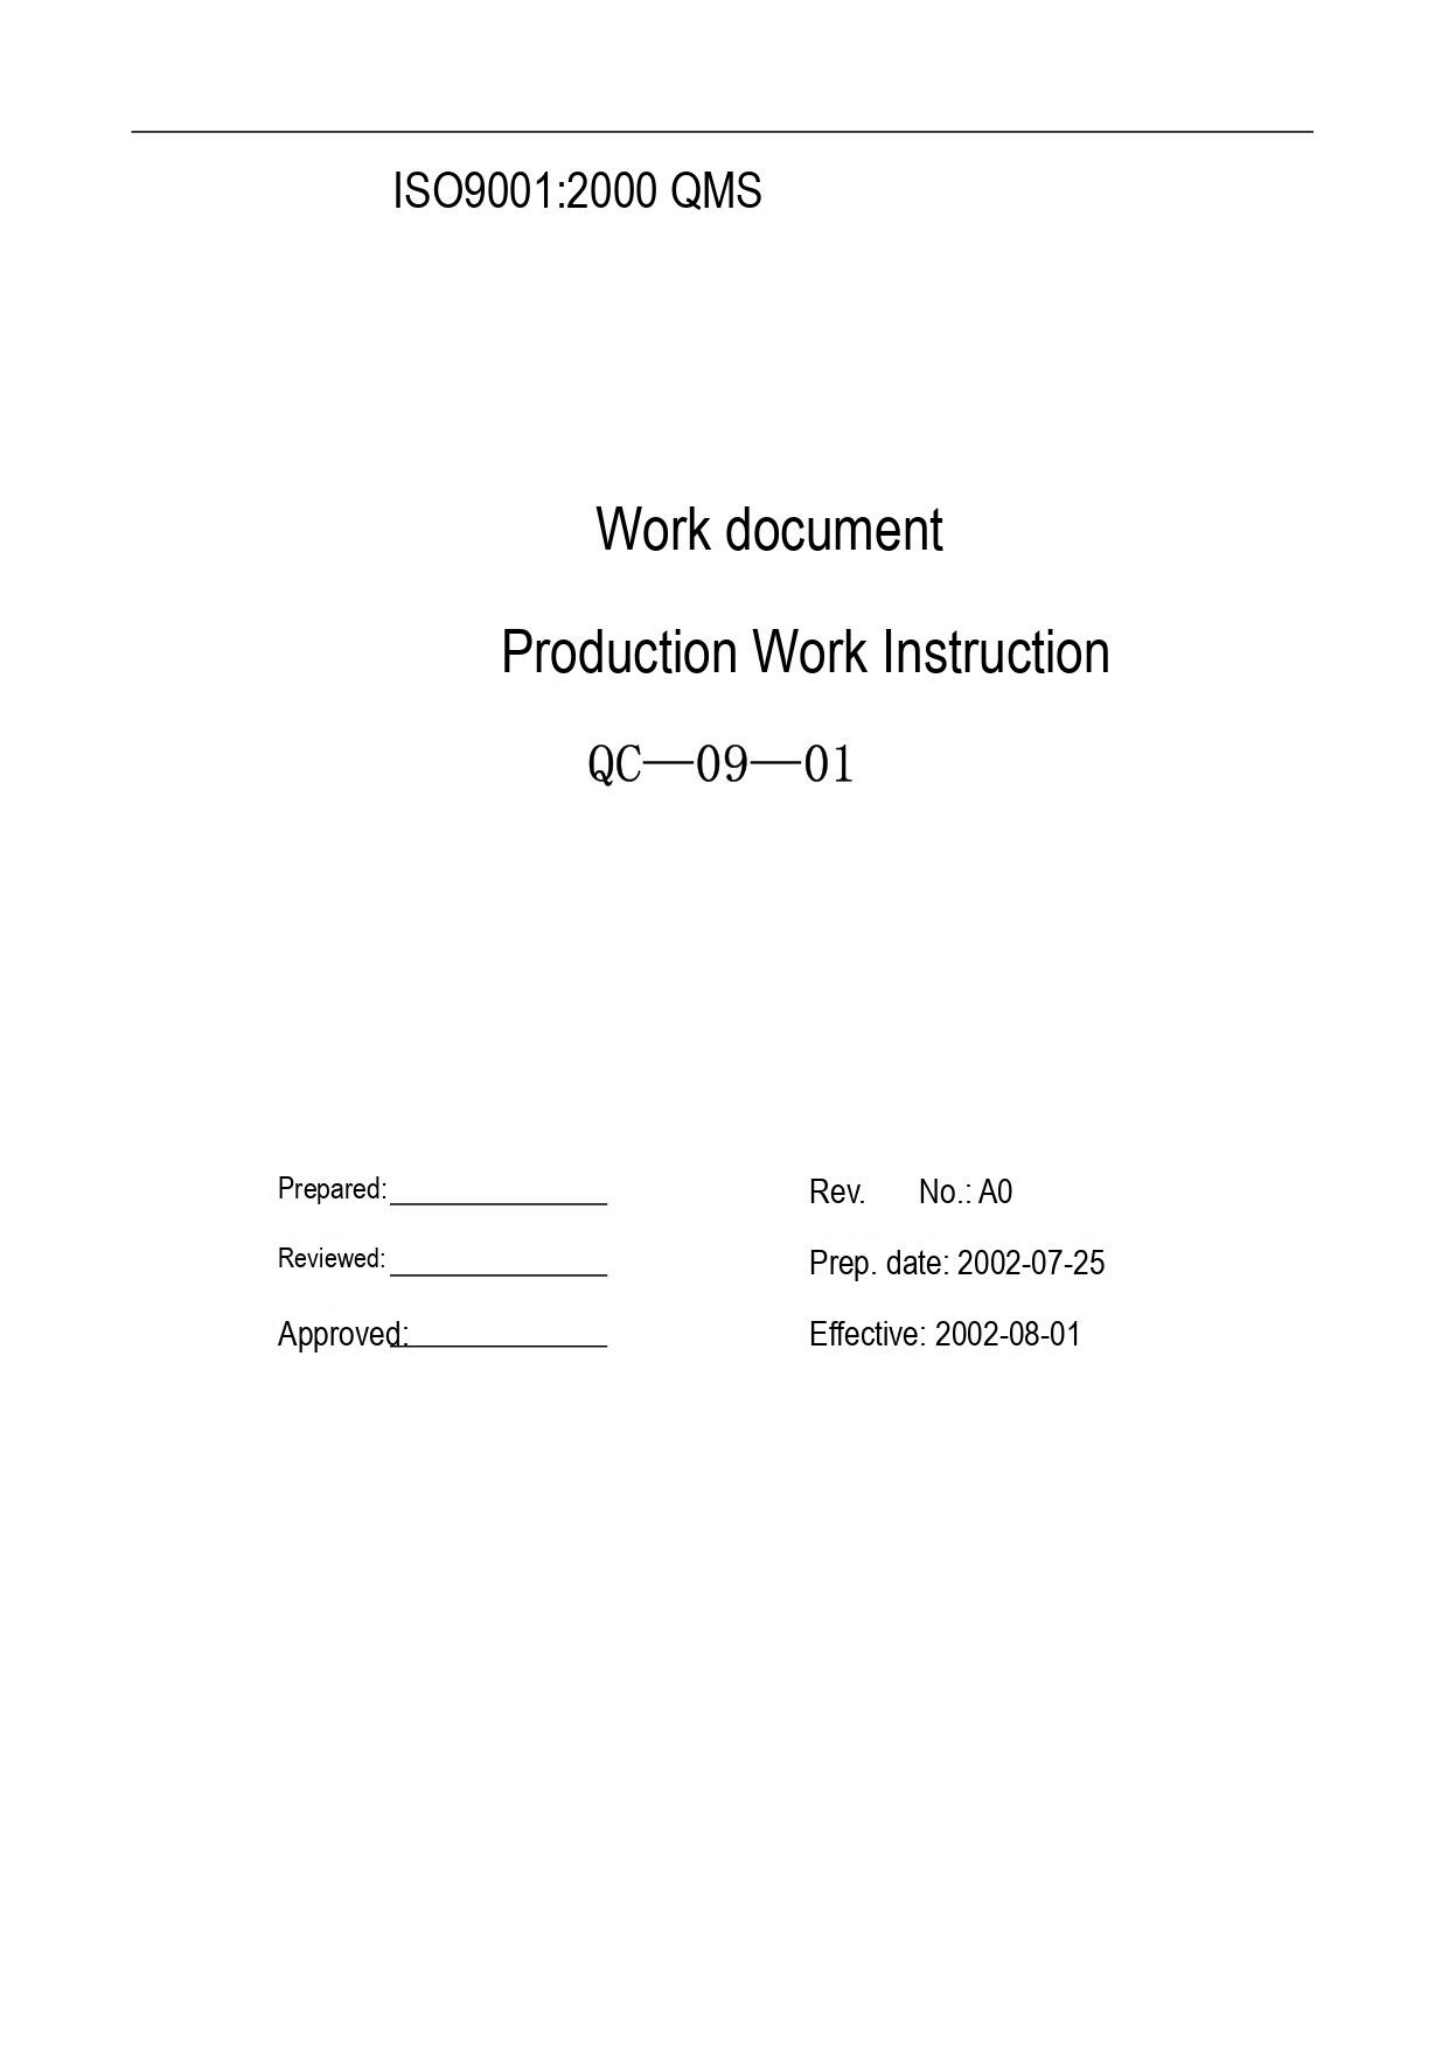ISO9001:2000 QMS

Work document

Production Work Instruction

QC—09—01

Prepared:_______________

Reviewed:_______________

Approved:_______________

Rev. No.: A0

Prep. date: 2002-07-25

Effective: 2002-08-01
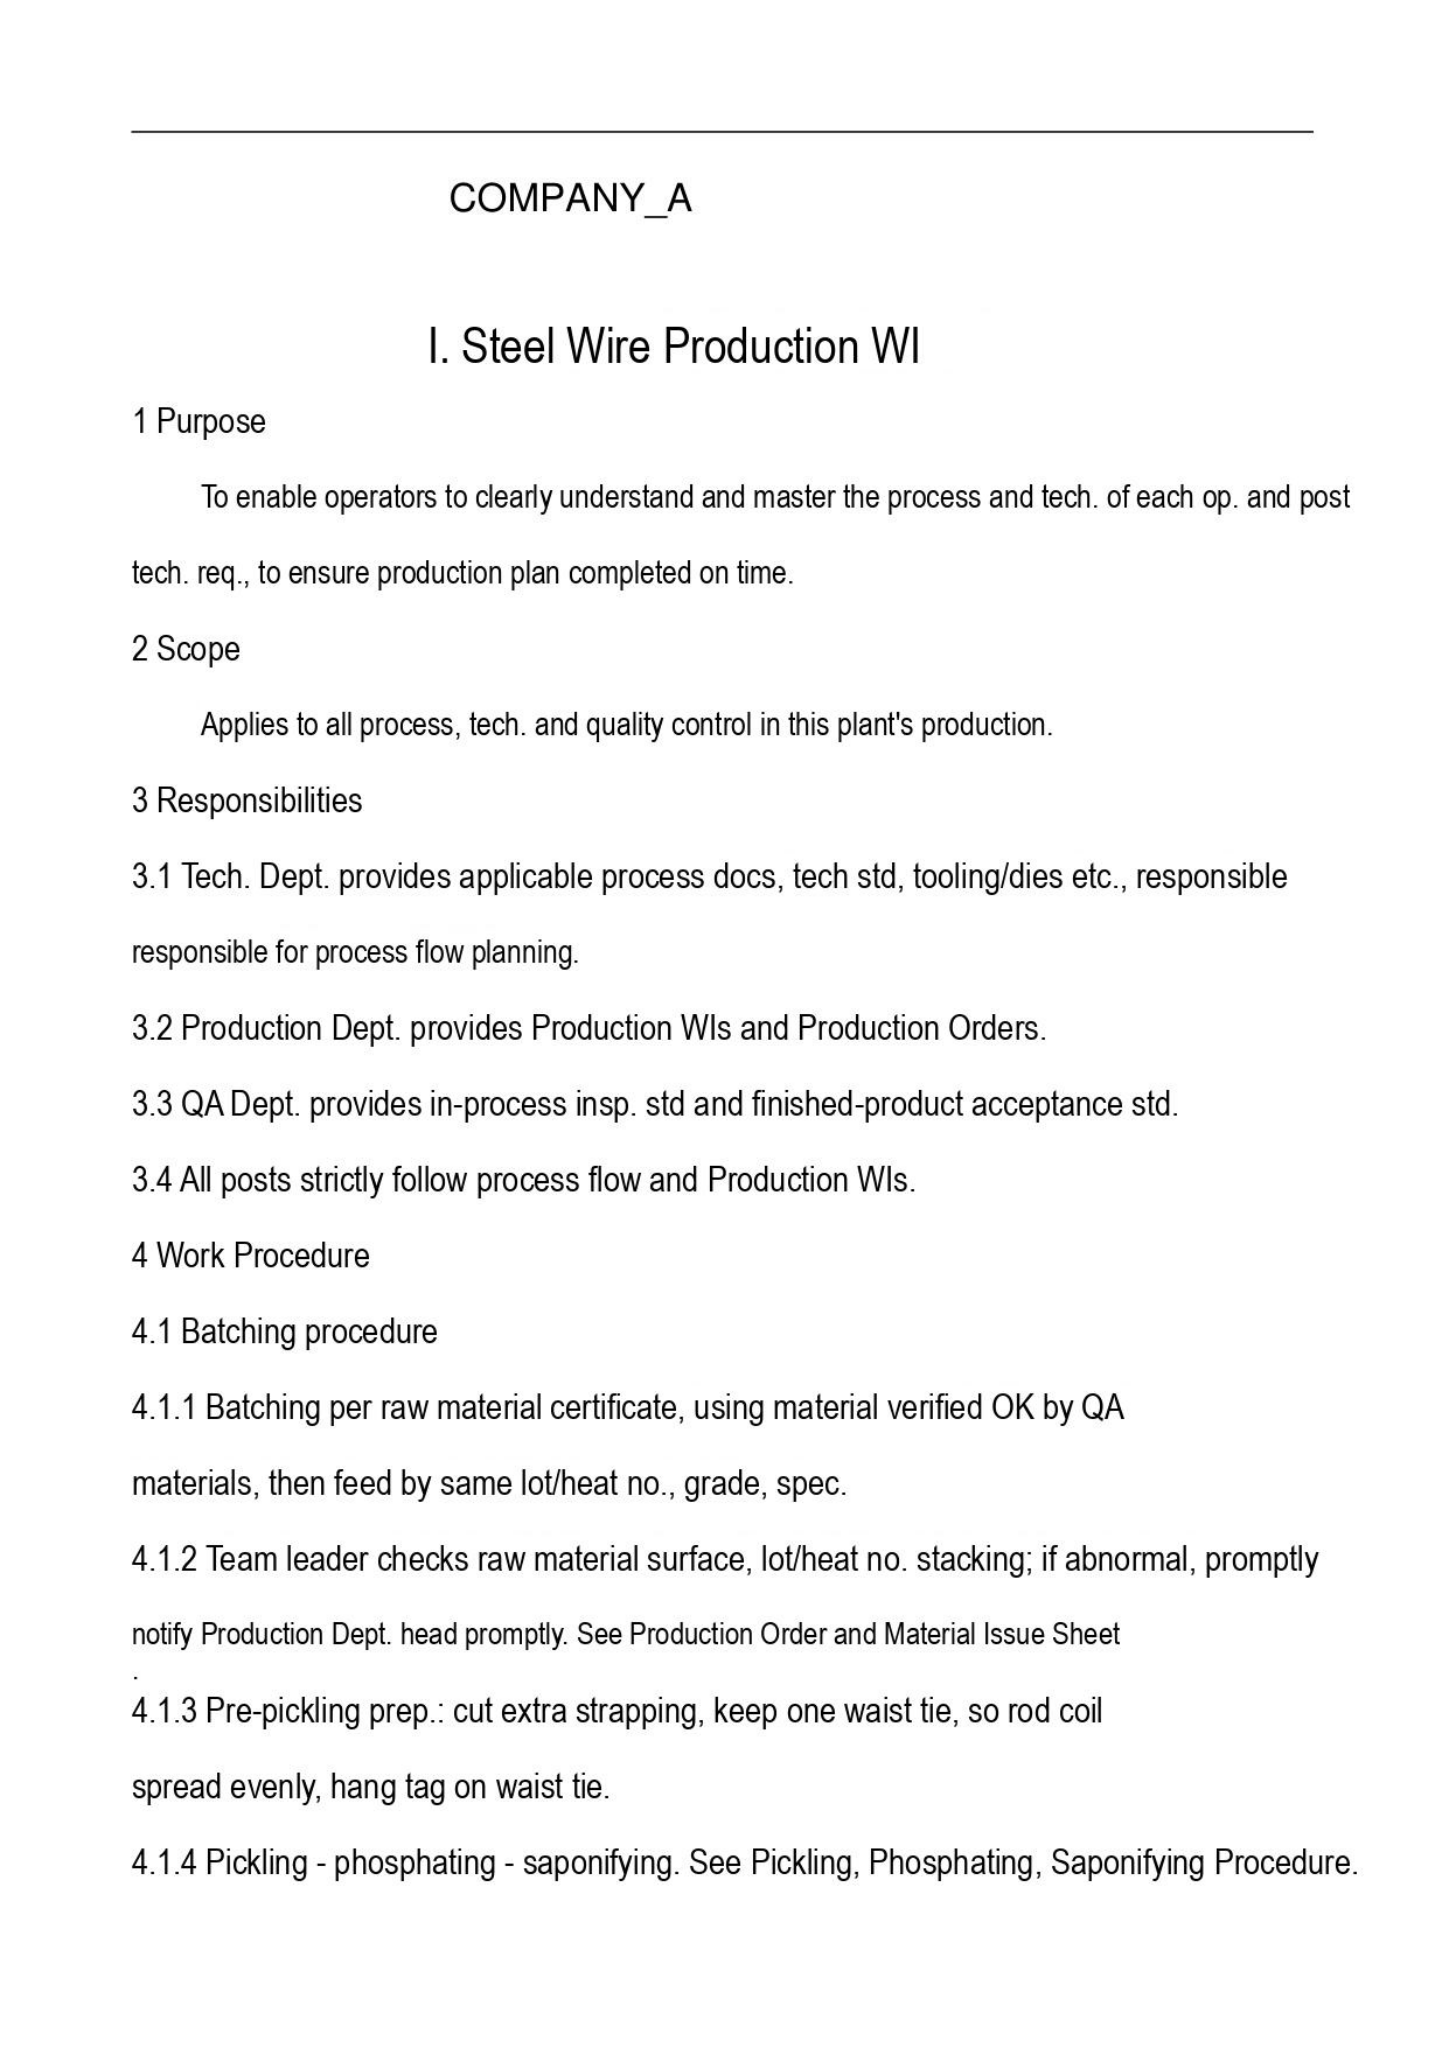COMPANY_A

I. Steel Wire Production WI

1 Purpose

To enable operators to clearly understand and master the process and tech. of each op. and post tech. req., to ensure production plan completed on time.

2 Scope

Applies to all process, tech. and quality control in this plant's production.

3 Responsibilities

3.1 Tech. Dept. provides applicable process docs, tech std, tooling/dies etc., responsible responsible for process flow planning.

3.2 Production Dept. provides Production WIs and Production Orders.

3.3 QA Dept. provides in-process insp. std and finished-product acceptance std.

3.4 All posts strictly follow process flow and Production WIs.

4 Work Procedure

4.1 Batching procedure

4.1.1 Batching per raw material certificate, using material verified OK by QA materials, then feed by same lot/heat no., grade, spec.

4.1.2 Team leader checks raw material surface, lot/heat no. stacking; if abnormal, promptly notify Production Dept. head promptly. See Production Order and Material Issue Sheet.

4.1.3 Pre-pickling prep.: cut extra strapping, keep one waist tie, so rod coil spread evenly, hang tag on waist tie.

4.1.4 Pickling - phosphating - saponifying. See Pickling, Phosphating, Saponifying Procedure.
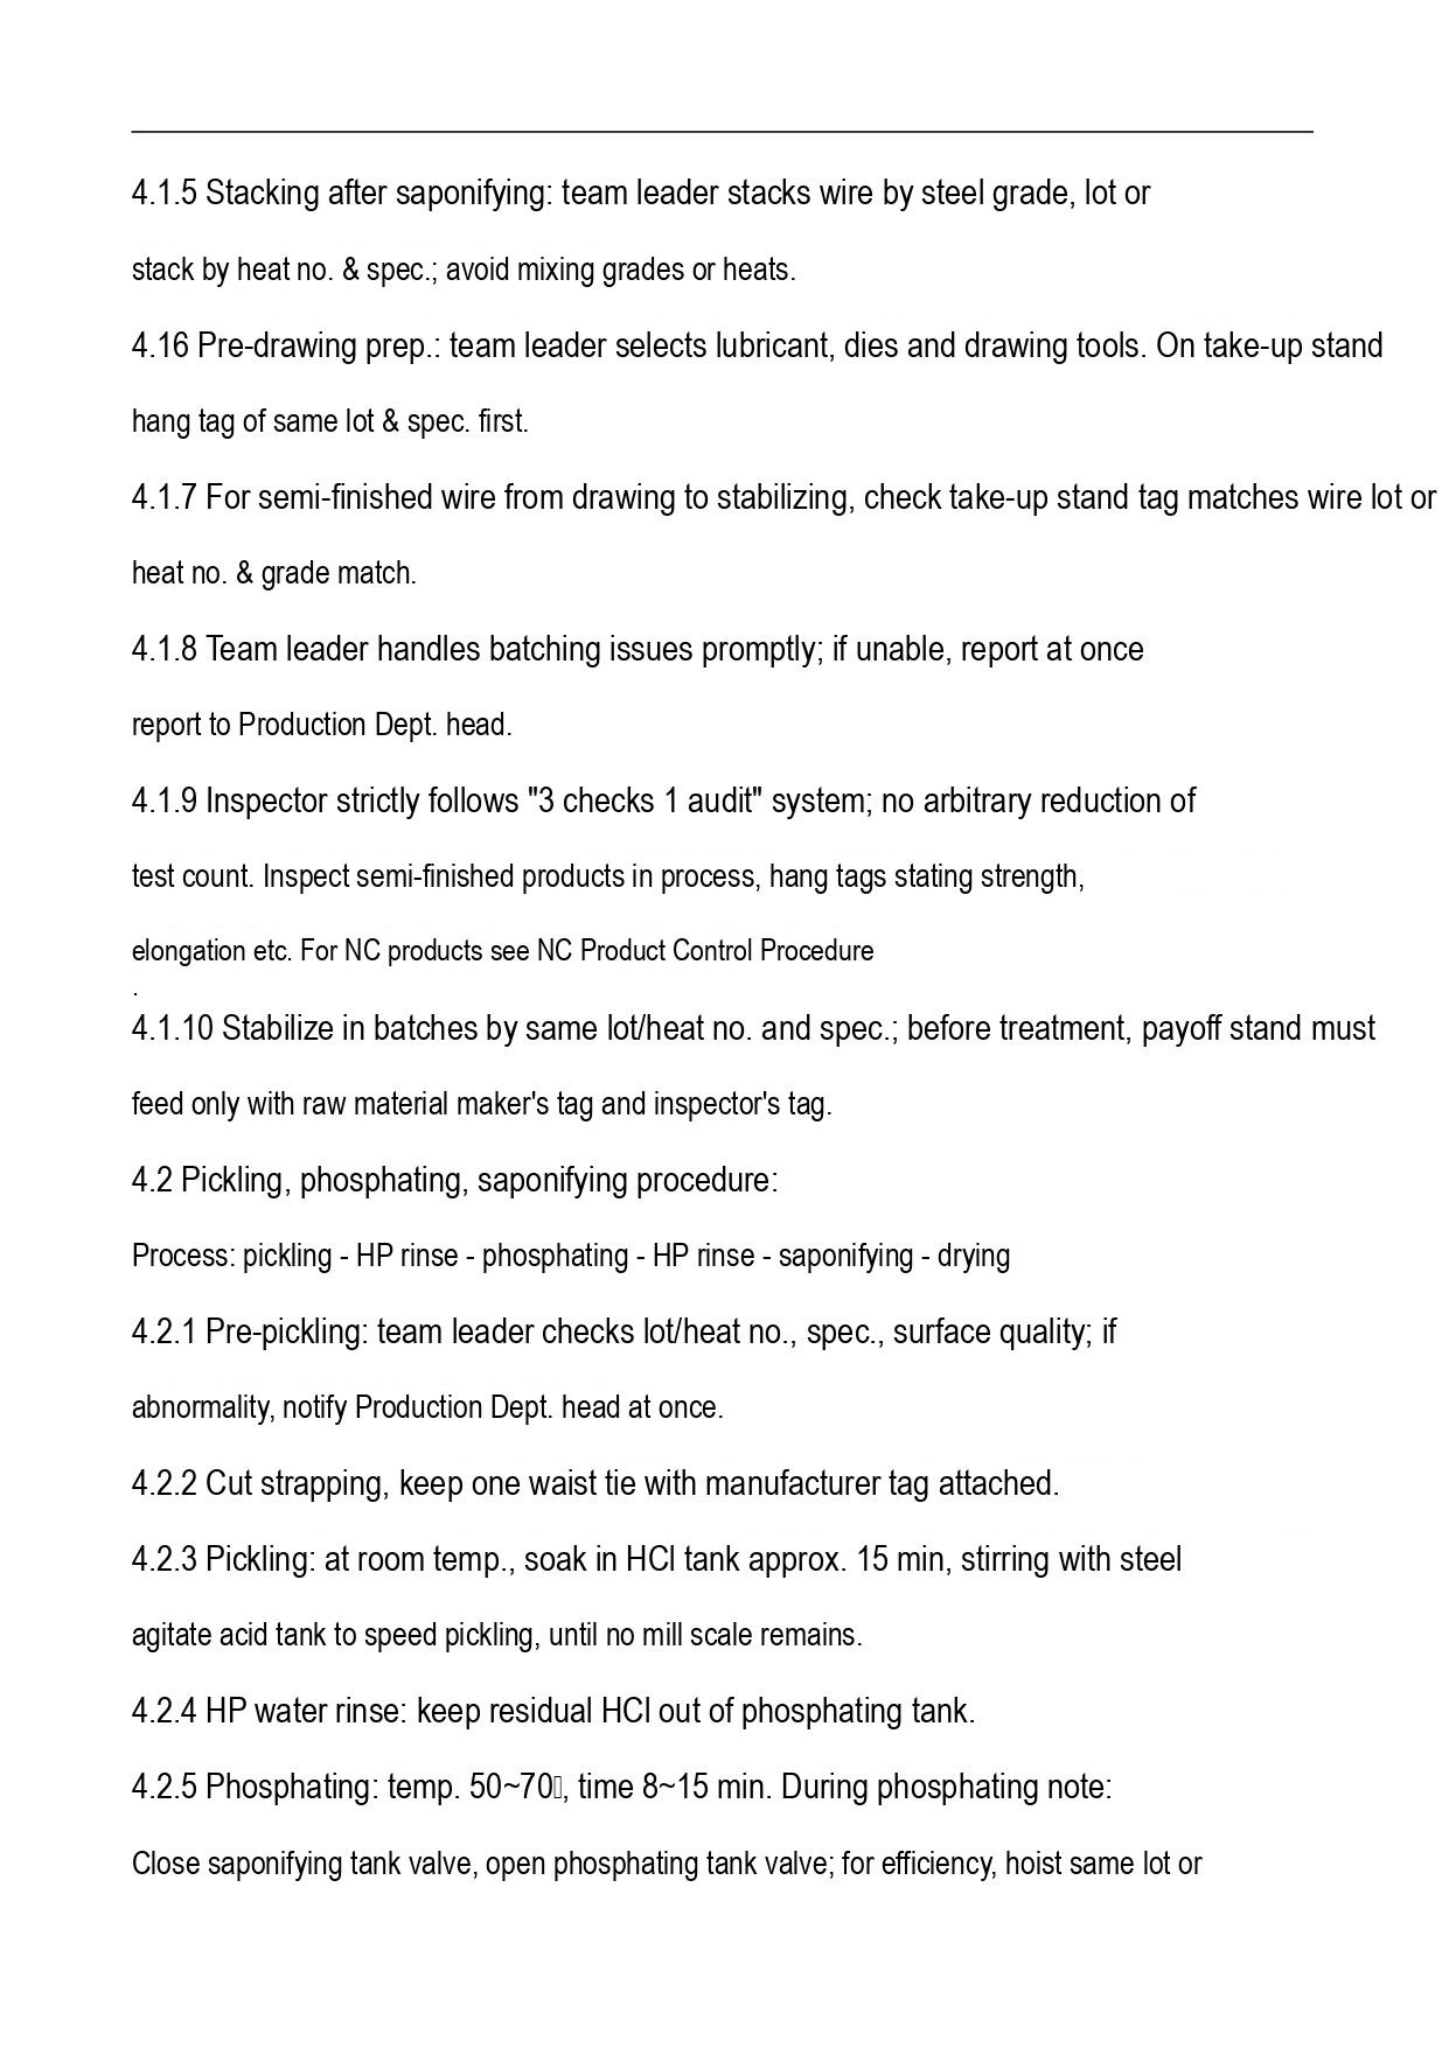4.1.5 Stacking after saponifying: team leader stacks wire by steel grade, lot or

stack by heat no. & spec.; avoid mixing grades or heats.

4.16 Pre-drawing prep.: team leader selects lubricant, dies and drawing tools. On take-up stand

hang tag of same lot & spec. first.

4.1.7 For semi-finished wire from drawing to stabilizing, check take-up stand tag matches wire lot or

heat no. & grade match.

4.1.8 Team leader handles batching issues promptly; if unable, report at once

report to Production Dept. head.

4.1.9 Inspector strictly follows "3 checks 1 audit" system; no arbitrary reduction of

test count. Inspect semi-finished products in process, hang tags stating strength,

elongation etc. For NC products see NC Product Control Procedure

.

4.1.10 Stabilize in batches by same lot/heat no. and spec.; before treatment, payoff stand must

feed only with raw material maker's tag and inspector's tag.

4.2 Pickling, phosphating, saponifying procedure:

Process: pickling - HP rinse - phosphating - HP rinse - saponifying - drying

4.2.1 Pre-pickling: team leader checks lot/heat no., spec., surface quality; if

abnormality, notify Production Dept. head at once.

4.2.2 Cut strapping, keep one waist tie with manufacturer tag attached.

4.2.3 Pickling: at room temp., soak in HCl tank approx. 15 min, stirring with steel

agitate acid tank to speed pickling, until no mill scale remains.

4.2.4 HP water rinse: keep residual HCl out of phosphating tank.

4.2.5 Phosphating: temp. 50~70, time 8~15 min. During phosphating note:

Close saponifying tank valve, open phosphating tank valve; for efficiency, hoist same lot or
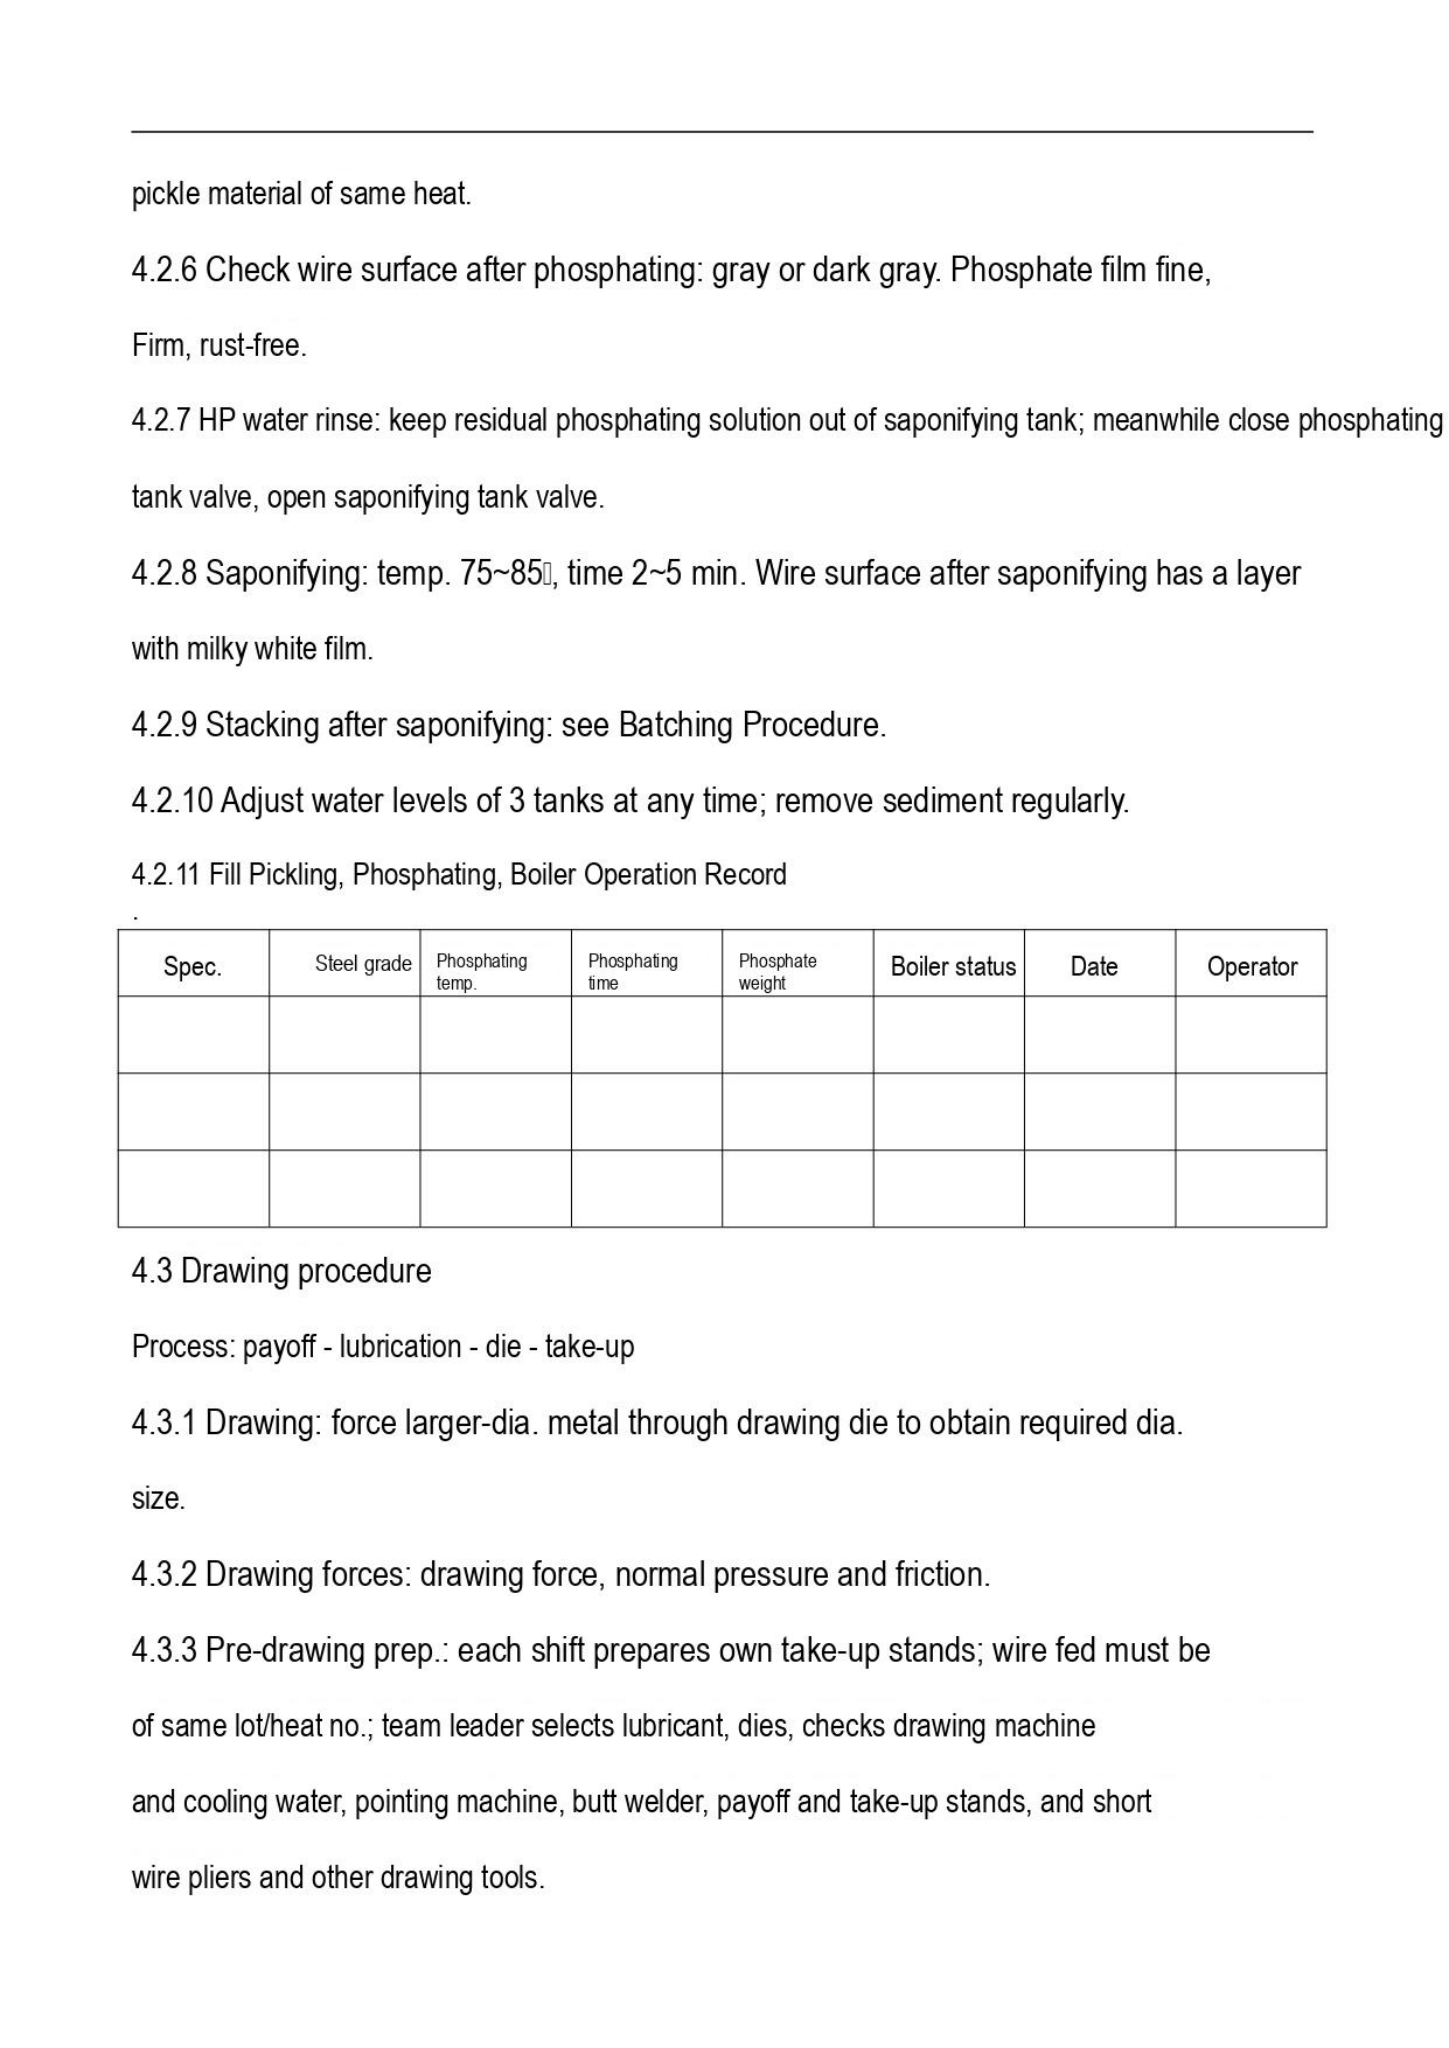pickle material of same heat.

4.2.6 Check wire surface after phosphating: gray or dark gray. Phosphate film fine,

Firm, rust-free.

4.2.7 HP water rinse: keep residual phosphating solution out of saponifying tank; meanwhile close phosphating

tank valve, open saponifying tank valve.

4.2.8 Saponifying: temp. 75~85, time 2~5 min. Wire surface after saponifying has a layer

with milky white film.

4.2.9 Stacking after saponifying: see Batching Procedure.

4.2.10 Adjust water levels of 3 tanks at any time; remove sediment regularly.

4.2.11 Fill Pickling, Phosphating, Boiler Operation Record

.

| Spec. | Steel grade | Phosphating temp. | Phosphating time | Phosphate weight | Boiler status | Date | Operator |
|---|---|---|---|---|---|---|---|
| | | | | | | | |
| | | | | | | | |
| | | | | | | | |

4.3 Drawing procedure

Process: payoff - lubrication - die - take-up

4.3.1 Drawing: force larger-dia. metal through drawing die to obtain required dia.

size.

4.3.2 Drawing forces: drawing force, normal pressure and friction.

4.3.3 Pre-drawing prep.: each shift prepares own take-up stands; wire fed must be

of same lot/heat no.; team leader selects lubricant, dies, checks drawing machine

and cooling water, pointing machine, butt welder, payoff and take-up stands, and short

wire pliers and other drawing tools.
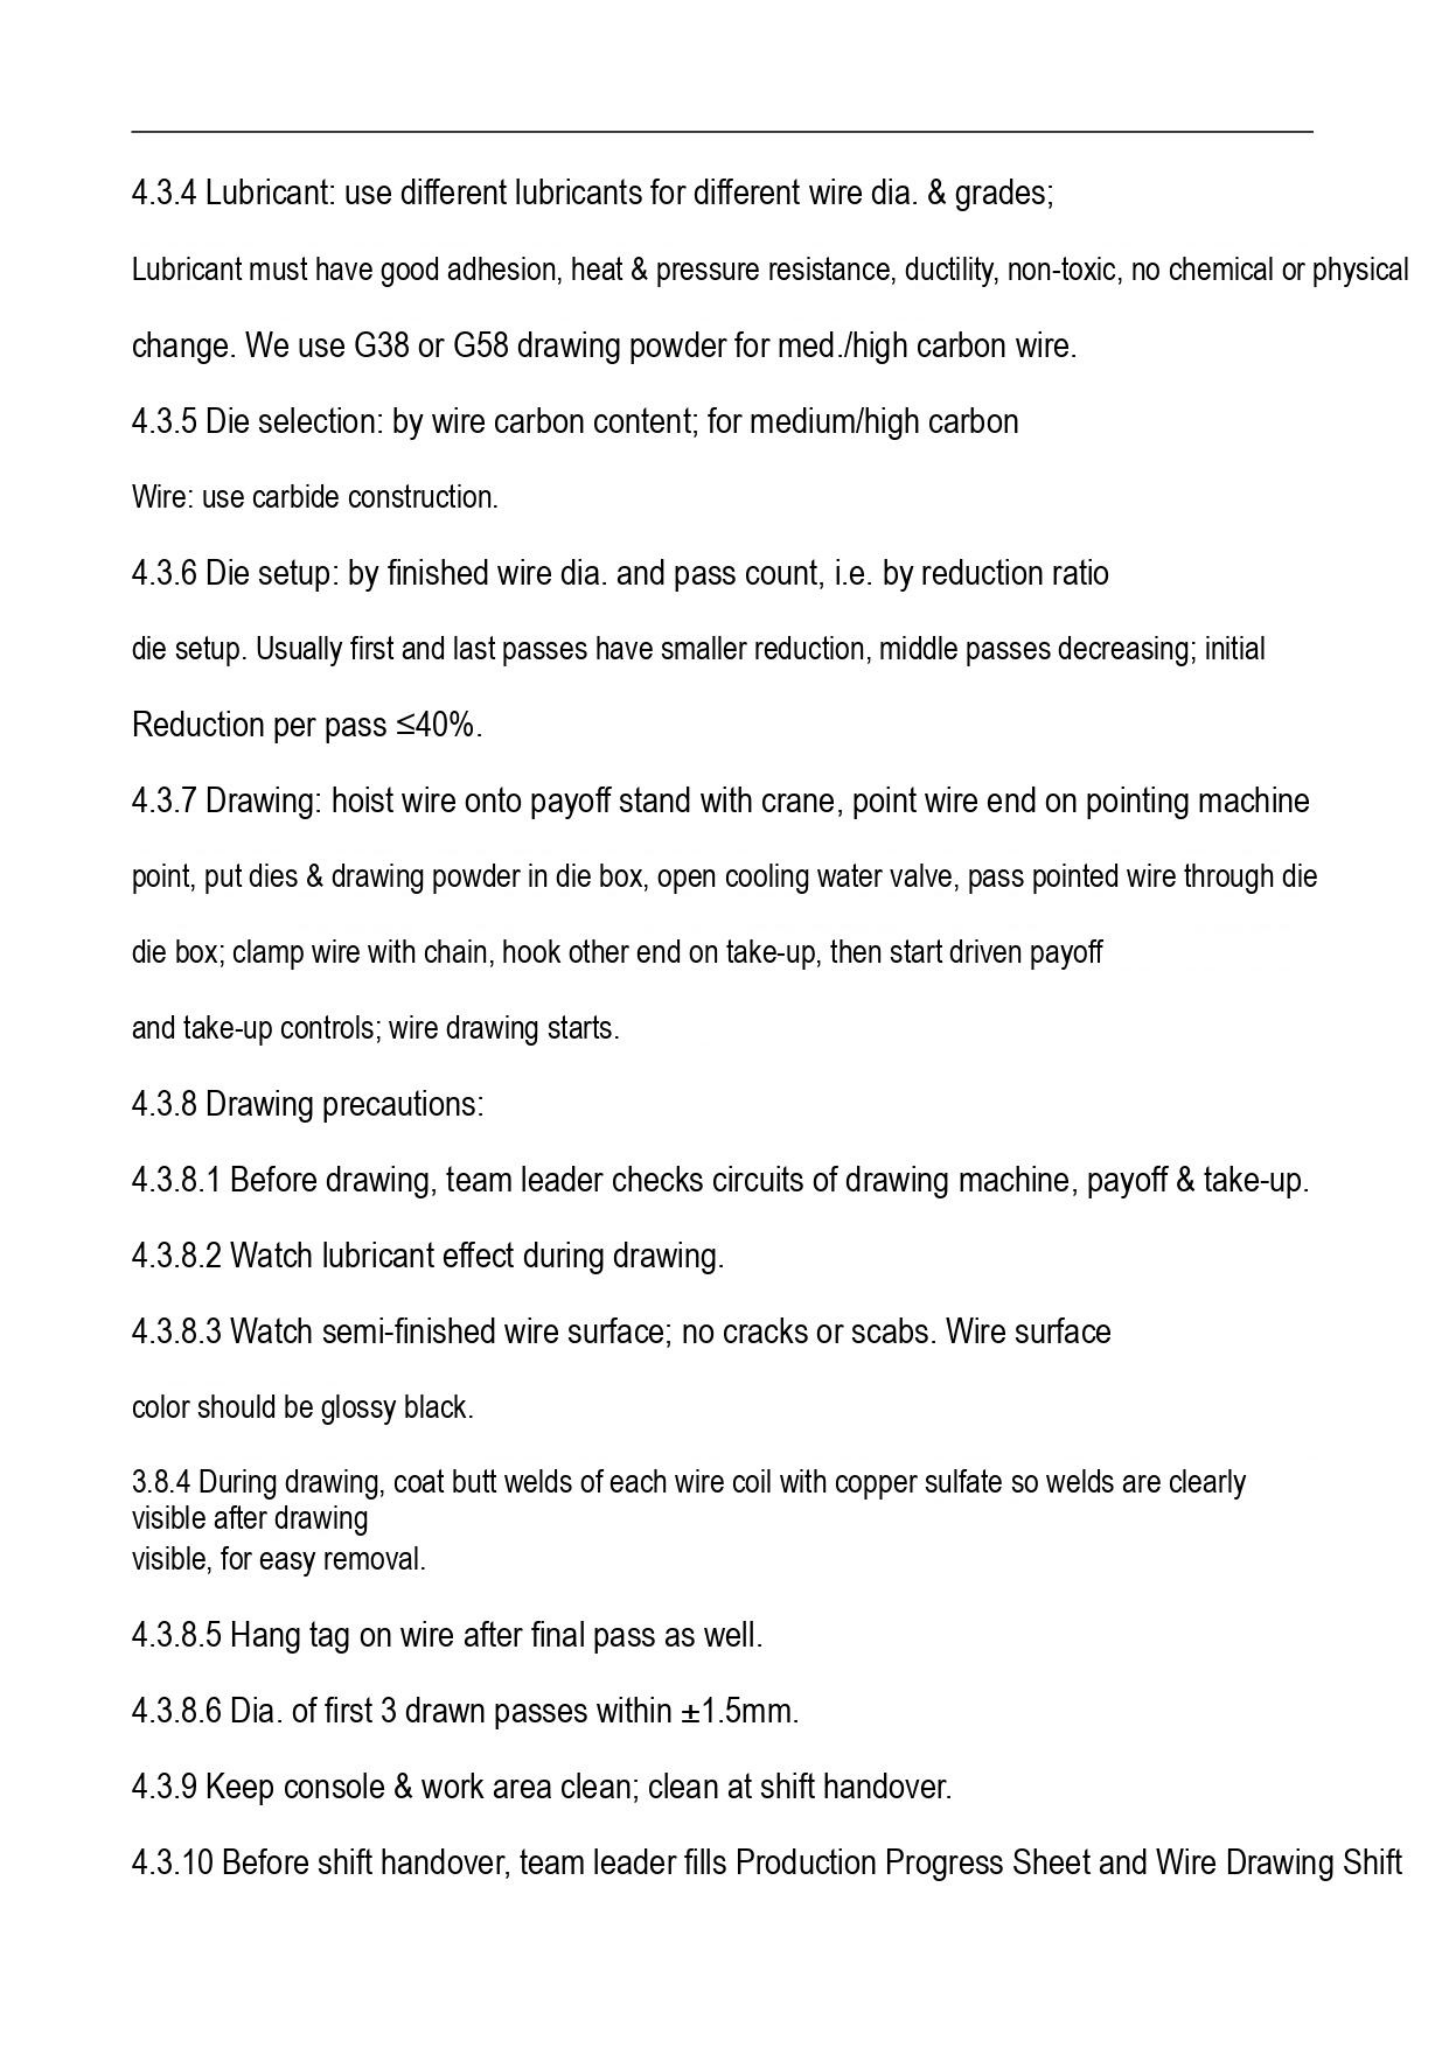4.3.4 Lubricant: use different lubricants for different wire dia. & grades;

Lubricant must have good adhesion, heat & pressure resistance, ductility, non-toxic, no chemical or physical

change. We use G38 or G58 drawing powder for med./high carbon wire.

4.3.5 Die selection: by wire carbon content; for medium/high carbon

Wire: use carbide construction.

4.3.6 Die setup: by finished wire dia. and pass count, i.e. by reduction ratio

die setup. Usually first and last passes have smaller reduction, middle passes decreasing; initial

Reduction per pass ≤40%.

4.3.7 Drawing: hoist wire onto payoff stand with crane, point wire end on pointing machine

point, put dies & drawing powder in die box, open cooling water valve, pass pointed wire through die

die box; clamp wire with chain, hook other end on take-up, then start driven payoff

and take-up controls; wire drawing starts.

4.3.8 Drawing precautions:

4.3.8.1 Before drawing, team leader checks circuits of drawing machine, payoff & take-up.

4.3.8.2 Watch lubricant effect during drawing.

4.3.8.3 Watch semi-finished wire surface; no cracks or scabs. Wire surface

color should be glossy black.

3.8.4 During drawing, coat butt welds of each wire coil with copper sulfate so welds are clearly
visible after drawing
visible, for easy removal.

4.3.8.5 Hang tag on wire after final pass as well.

4.3.8.6 Dia. of first 3 drawn passes within ±1.5mm.

4.3.9 Keep console & work area clean; clean at shift handover.

4.3.10 Before shift handover, team leader fills Production Progress Sheet and Wire Drawing Shift
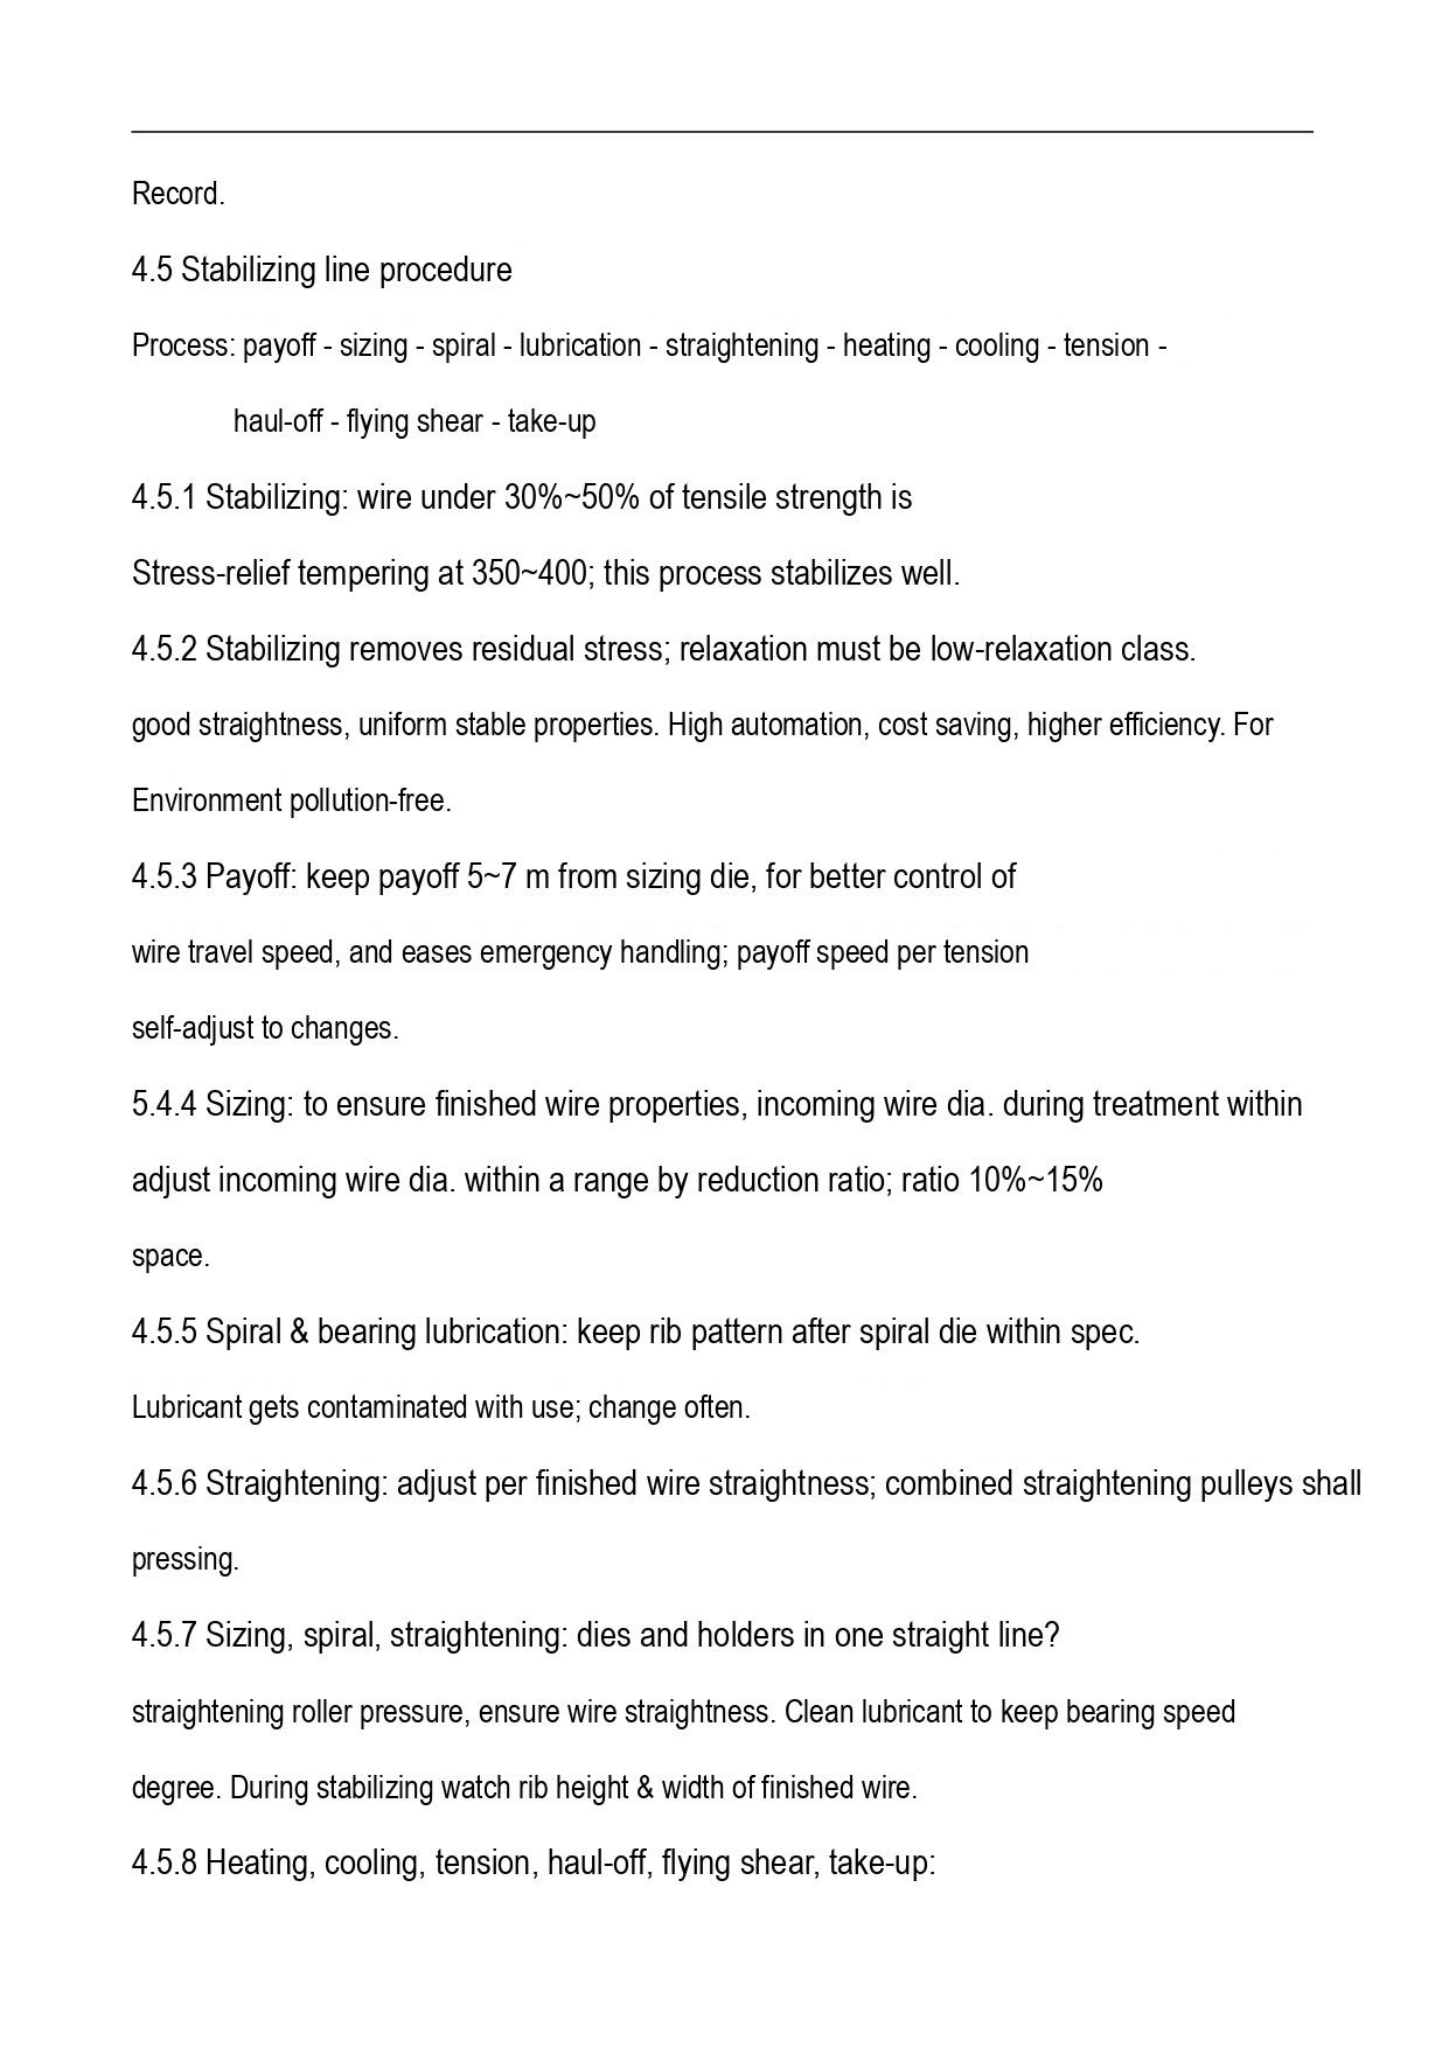Record.

4.5 Stabilizing line procedure

Process: payoff - sizing - spiral - lubrication - straightening - heating - cooling - tension -

haul-off - flying shear - take-up

4.5.1 Stabilizing: wire under 30%~50% of tensile strength is

Stress-relief tempering at 350~400; this process stabilizes well.

4.5.2 Stabilizing removes residual stress; relaxation must be low-relaxation class.

good straightness, uniform stable properties. High automation, cost saving, higher efficiency. For

Environment pollution-free.

4.5.3 Payoff: keep payoff 5~7 m from sizing die, for better control of

wire travel speed, and eases emergency handling; payoff speed per tension

self-adjust to changes.

5.4.4 Sizing: to ensure finished wire properties, incoming wire dia. during treatment within

adjust incoming wire dia. within a range by reduction ratio; ratio 10%~15%

space.

4.5.5 Spiral & bearing lubrication: keep rib pattern after spiral die within spec.

Lubricant gets contaminated with use; change often.

4.5.6 Straightening: adjust per finished wire straightness; combined straightening pulleys shall

pressing.

4.5.7 Sizing, spiral, straightening: dies and holders in one straight line?

straightening roller pressure, ensure wire straightness. Clean lubricant to keep bearing speed

degree. During stabilizing watch rib height & width of finished wire.

4.5.8 Heating, cooling, tension, haul-off, flying shear, take-up:
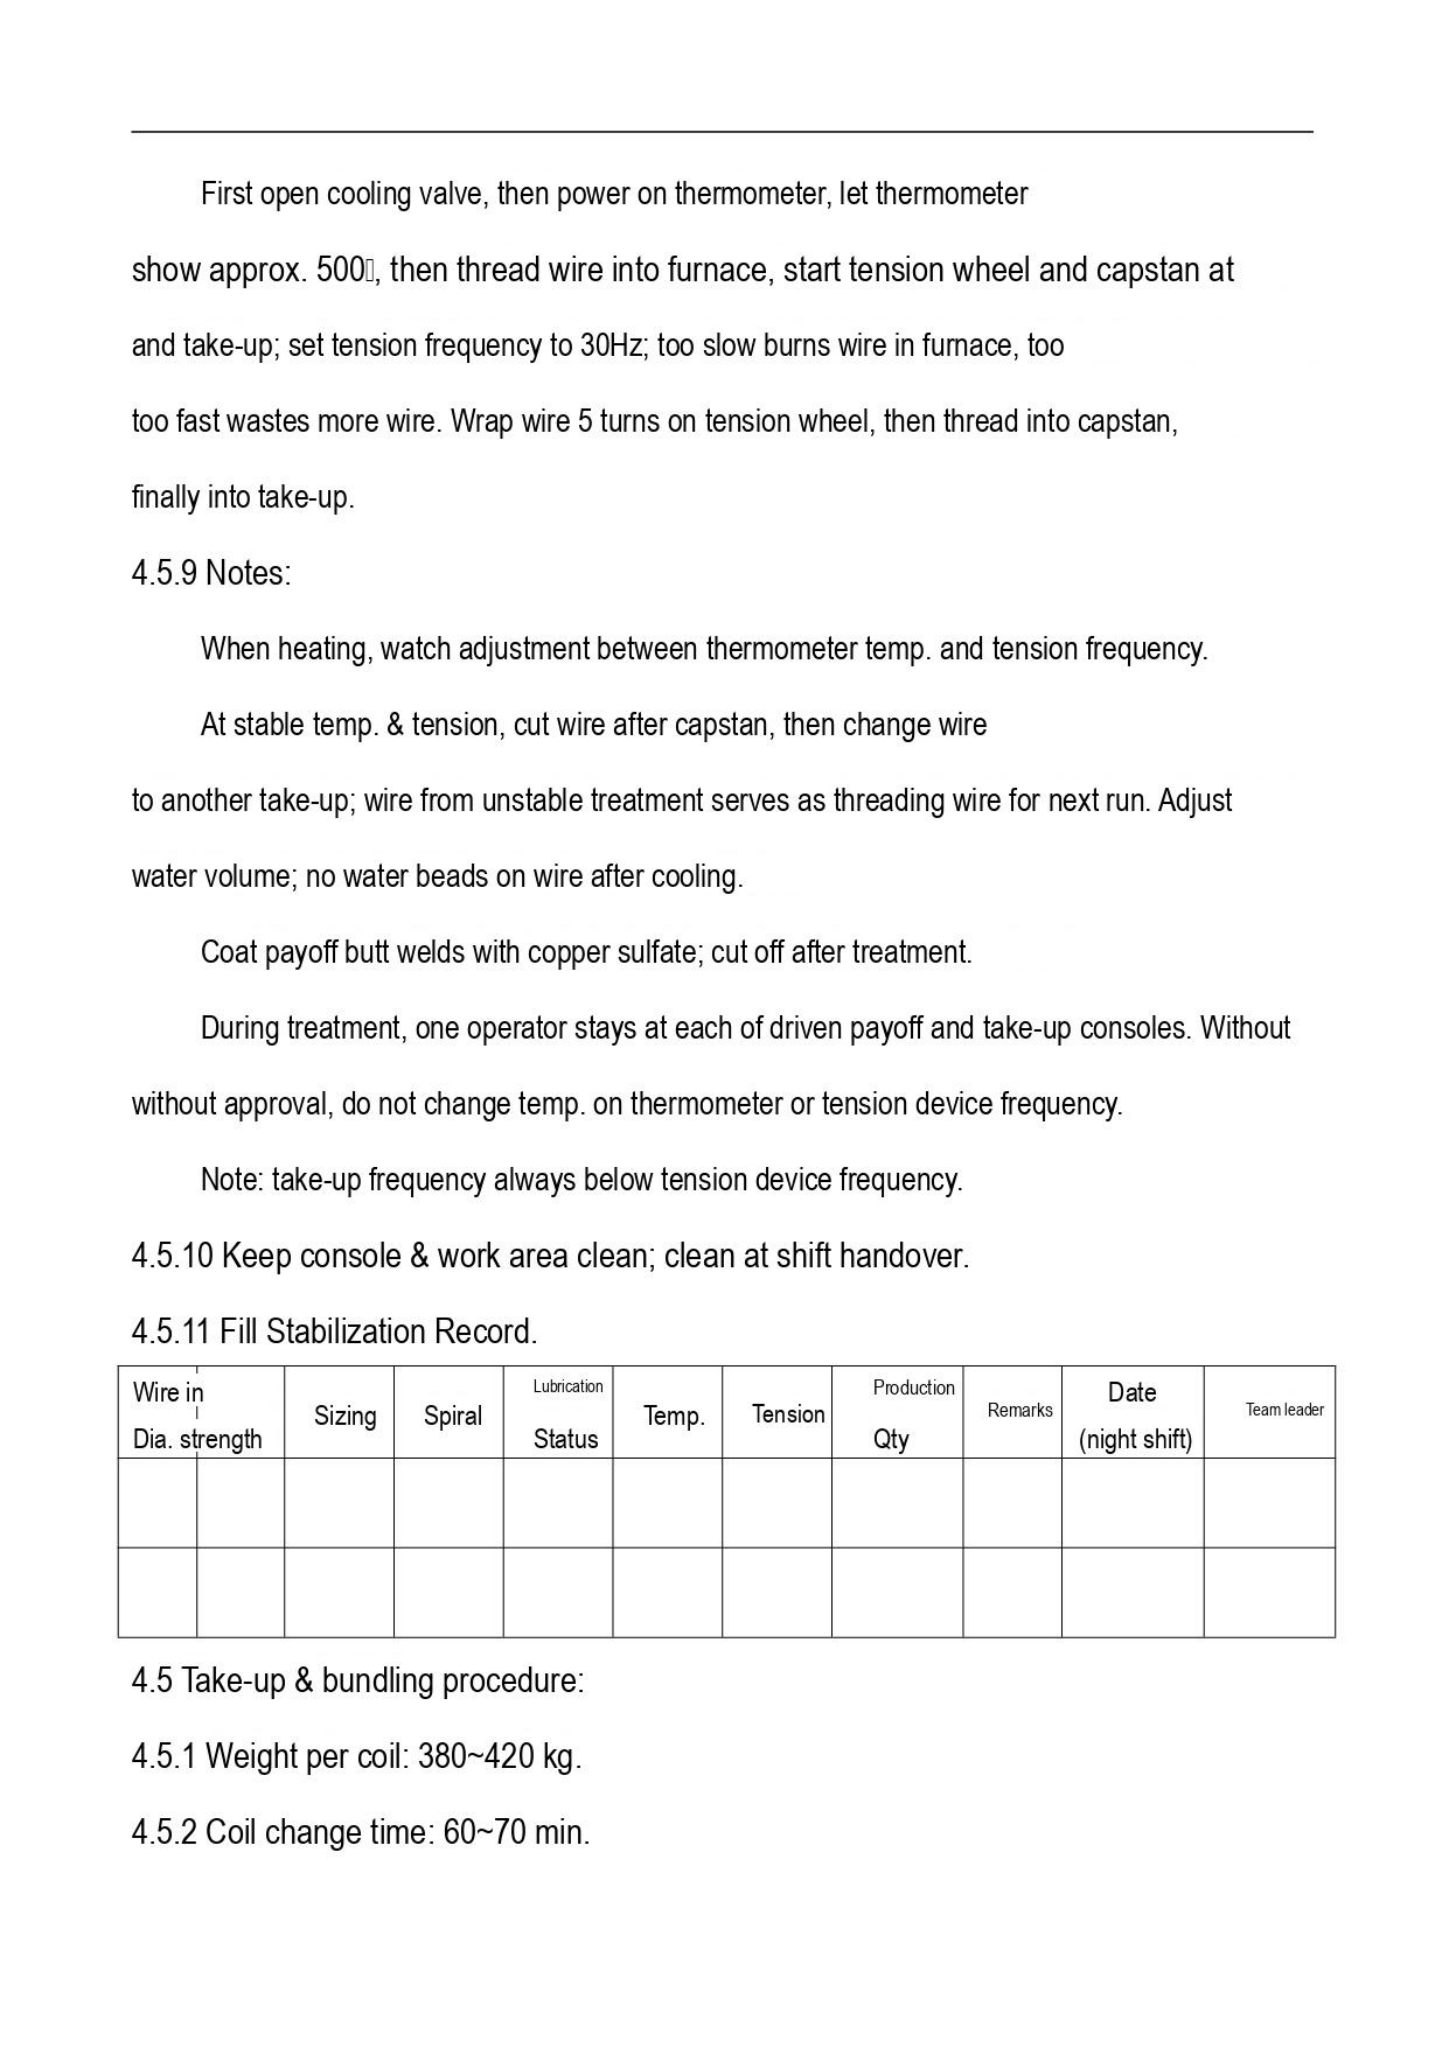First open cooling valve, then power on thermometer, let thermometer

show approx. 500, then thread wire into furnace, start tension wheel and capstan at

and take-up; set tension frequency to 30Hz; too slow burns wire in furnace, too

too fast wastes more wire. Wrap wire 5 turns on tension wheel, then thread into capstan,

finally into take-up.

4.5.9 Notes:

When heating, watch adjustment between thermometer temp. and tension frequency.

At stable temp. & tension, cut wire after capstan, then change wire

to another take-up; wire from unstable treatment serves as threading wire for next run. Adjust

water volume; no water beads on wire after cooling.

Coat payoff butt welds with copper sulfate; cut off after treatment.

During treatment, one operator stays at each of driven payoff and take-up consoles. Without

without approval, do not change temp. on thermometer or tension device frequency.

Note: take-up frequency always below tension device frequency.

4.5.10 Keep console & work area clean; clean at shift handover.

4.5.11 Fill Stabilization Record.

| Wire Dia. | in strength | Sizing | Spiral | Lubrication Status | Temp. | Tension | Production Qty | Remarks | Date (night shift) | Team leader |
|---|---|---|---|---|---|---|---|---|---|---|
| | | | | | | | | | | |
| | | | | | | | | | | |

4.5 Take-up & bundling procedure:

4.5.1 Weight per coil: 380~420 kg.

4.5.2 Coil change time: 60~70 min.